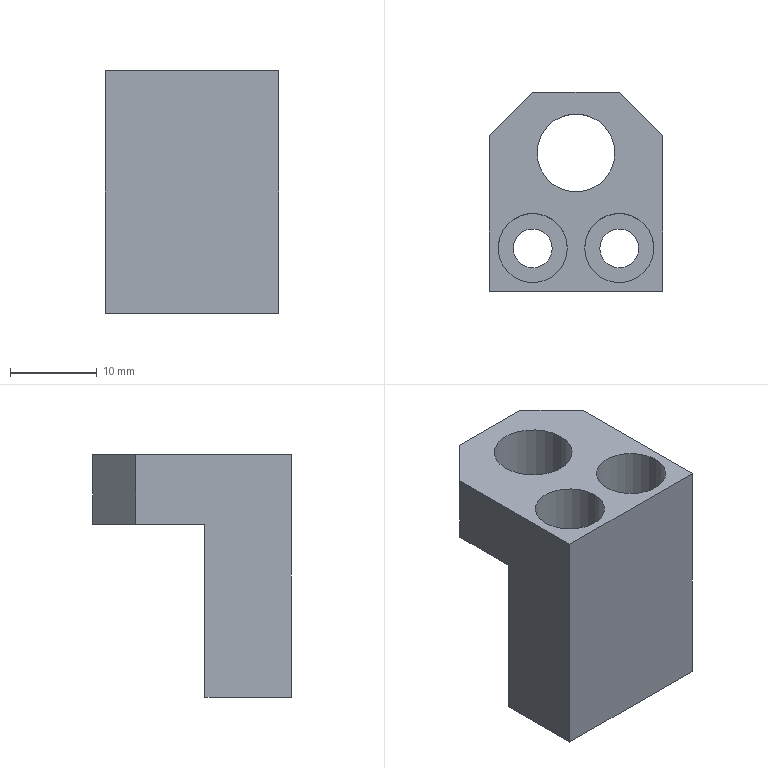Part | STEP file | D10 | 1 solid | 22 faces | box 20 x 23 x 28 mm | volume 4706 mm3 | plane 12 | cylinder 10 | commonest cylinder face diameters 4.5 x4 8 x4 9 x2